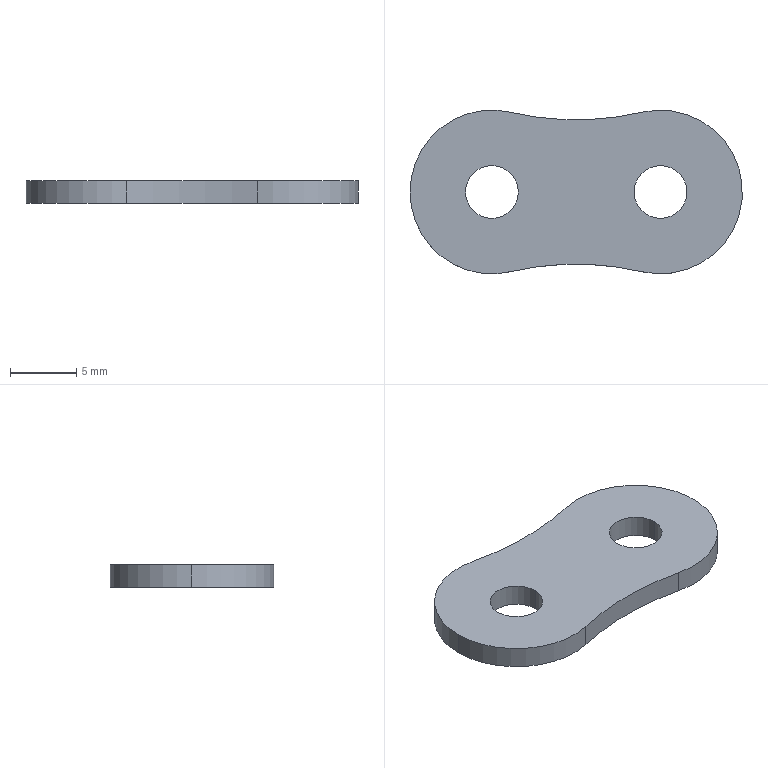Part | SolidWorks | features Cut 1, Extrusion 1 | 1 solid | 11 faces | box 25.03 x 12.33 x 1.665 mm | volume 399.679 mm3 | cylinder 9 | plane 2 | commonest cylinder face diameters 3.98 x4 12.33 x3 43.376 x2
STEP:
#1=CARTESIAN_POINT('',(4.36,0.,0.));
#2=VERTEX_POINT('',#1);
#3=CARTESIAN_POINT('',(8.34,0.,0.));
#4=VERTEX_POINT('',#3);
#5=CARTESIAN_POINT('',(6.35,0.,0.));
#6=DIRECTION('',(0.,0.,1.));
#7=DIRECTION('',(1.,0.,0.));
#8=AXIS2_PLACEMENT_3D('',#5,#6,#7);
#9=CIRCLE('',#8,1.99);
#10=EDGE_CURVE('',#2,#4,#9,.T.);
#11=ORIENTED_EDGE('',*,*,#10,.F.);
#12=CARTESIAN_POINT('',(4.36,0.,1.665));
#13=VERTEX_POINT('',#12);
#14=CARTESIAN_POINT('',(4.36,0.,0.));
#15=DIRECTION('',(0.,0.,1.));
#16=VECTOR('',#15,1000.);
#17=LINE('',#14,#16);
#18=EDGE_CURVE('',#2,#13,#17,.T.);
#19=ORIENTED_EDGE('',*,*,#18,.T.);
#20=CARTESIAN_POINT('',(8.34,0.,1.665));
#21=VERTEX_POINT('',#20);
#22=CARTESIAN_POINT('',(6.35,0.,1.665));
#23=DIRECTION('',(0.,0.,1.));
#24=DIRECTION('',(1.,0.,0.));
#25=AXIS2_PLACEMENT_3D('',#22,#23,#24);
#26=CIRCLE('',#25,1.99);
#27=EDGE_CURVE('',#13,#21,#26,.T.);
#28=ORIENTED_EDGE('',*,*,#27,.T.);
#29=CARTESIAN_POINT('',(8.34,0.,0.));
#30=DIRECTION('',(0.,0.,1.));
#31=VECTOR('',#30,1000.);
#32=LINE('',#29,#31);
#33=EDGE_CURVE('',#4,#21,#32,.T.);
#34=ORIENTED_EDGE('',*,*,#33,.F.);
#35=EDGE_LOOP('',(#11,#19,#28,#34));
#36=FACE_OUTER_BOUND('',#35,.T.);
#37=CARTESIAN_POINT('',(6.35,0.,0.));
#38=DIRECTION('',(0.,0.,1.));
#39=DIRECTION('',(1.,0.,0.));
#40=AXIS2_PLACEMENT_3D('',#37,#38,#39);
#41=CYLINDRICAL_SURFACE('',#40,1.99);
#42=ADVANCED_FACE('',(#36),#41,.F.);
#43=CARTESIAN_POINT('',(-8.34,0.,0.));
#44=VERTEX_POINT('',#43);
#45=CARTESIAN_POINT('',(-4.36,0.,0.));
#46=VERTEX_POINT('',#45);
#47=CARTESIAN_POINT('',(-6.35,0.,0.));
#48=DIRECTION('',(0.,0.,1.));
#49=DIRECTION('',(1.,0.,0.));
#50=AXIS2_PLACEMENT_3D('',#47,#48,#49);
#51=CIRCLE('',#50,1.99);
#52=EDGE_CURVE('',#44,#46,#51,.T.);
#53=ORIENTED_EDGE('',*,*,#52,.F.);
#54=CARTESIAN_POINT('',(-8.34,0.,1.665));
#55=VERTEX_POINT('',#54);
#56=CARTESIAN_POINT('',(-8.34,0.,0.));
#57=DIRECTION('',(0.,0.,1.));
#58=VECTOR('',#57,1000.);
#59=LINE('',#56,#58);
#60=EDGE_CURVE('',#44,#55,#59,.T.);
#61=ORIENTED_EDGE('',*,*,#60,.T.);
#62=CARTESIAN_POINT('',(-4.36,0.,1.665));
#63=VERTEX_POINT('',#62);
#64=CARTESIAN_POINT('',(-6.35,0.,1.665));
#65=DIRECTION('',(0.,0.,1.));
#66=DIRECTION('',(1.,0.,0.));
#67=AXIS2_PLACEMENT_3D('',#64,#65,#66);
#68=CIRCLE('',#67,1.99);
#69=EDGE_CURVE('',#55,#63,#68,.T.);
#70=ORIENTED_EDGE('',*,*,#69,.T.);
#71=CARTESIAN_POINT('',(-4.36,0.,0.));
#72=DIRECTION('',(0.,0.,1.));
#73=VECTOR('',#72,1000.);
#74=LINE('',#71,#73);
#75=EDGE_CURVE('',#46,#63,#74,.T.);
#76=ORIENTED_EDGE('',*,*,#75,.F.);
#77=EDGE_LOOP('',(#53,#61,#70,#76));
#78=FACE_OUTER_BOUND('',#77,.T.);
#79=CARTESIAN_POINT('',(-6.35,0.,0.));
#80=DIRECTION('',(0.,0.,1.));
#81=DIRECTION('',(1.,0.,0.));
#82=AXIS2_PLACEMENT_3D('',#79,#80,#81);
#83=CYLINDRICAL_SURFACE('',#82,1.99);
#84=ADVANCED_FACE('',(#78),#83,.F.);
#85=CARTESIAN_POINT('',(-12.515,0.,1.665));
#86=VERTEX_POINT('',#85);
#87=CARTESIAN_POINT('',(-4.944,-6.003,1.665));
#88=VERTEX_POINT('',#87);
#89=CARTESIAN_POINT('',(-6.35,0.,1.665));
#90=DIRECTION('',(0.,0.,1.));
#91=DIRECTION('',(1.,0.,0.));
#92=AXIS2_PLACEMENT_3D('',#89,#90,#91);
#93=CIRCLE('',#92,6.165);
#94=EDGE_CURVE('',#86,#88,#93,.T.);
#95=ORIENTED_EDGE('',*,*,#94,.F.);
#96=CARTESIAN_POINT('',(-12.515,0.,0.));
#97=VERTEX_POINT('',#96);
#98=CARTESIAN_POINT('',(-12.515,0.,1.665));
#99=DIRECTION('',(0.,0.,-1.));
#100=VECTOR('',#99,1000.);
#101=LINE('',#98,#100);
#102=EDGE_CURVE('',#86,#97,#101,.T.);
#103=ORIENTED_EDGE('',*,*,#102,.T.);
#104=CARTESIAN_POINT('',(-4.944,-6.003,0.));
#105=VERTEX_POINT('',#104);
#106=CARTESIAN_POINT('',(-6.35,0.,0.));
#107=DIRECTION('',(0.,0.,1.));
#108=DIRECTION('',(1.,0.,0.));
#109=AXIS2_PLACEMENT_3D('',#106,#107,#108);
#110=CIRCLE('',#109,6.165);
#111=EDGE_CURVE('',#97,#105,#110,.T.);
#112=ORIENTED_EDGE('',*,*,#111,.T.);
#113=CARTESIAN_POINT('',(-4.944,-6.003,1.665));
#114=DIRECTION('',(0.,0.,-1.));
#115=VECTOR('',#114,1000.);
#116=LINE('',#113,#115);
#117=EDGE_CURVE('',#88,#105,#116,.T.);
#118=ORIENTED_EDGE('',*,*,#117,.F.);
#119=EDGE_LOOP('',(#95,#103,#112,#118));
#120=FACE_OUTER_BOUND('',#119,.T.);
#121=CARTESIAN_POINT('',(-6.35,0.,1.665));
#122=DIRECTION('',(0.,0.,-1.));
#123=DIRECTION('',(-1.,0.,0.));
#124=AXIS2_PLACEMENT_3D('',#121,#122,#123);
#125=CYLINDRICAL_SURFACE('',#124,6.165);
#126=ADVANCED_FACE('',(#120),#125,.T.);
#127=CARTESIAN_POINT('',(4.944,-6.003,0.));
#128=VERTEX_POINT('',#127);
#129=CARTESIAN_POINT('',(0.,-27.12,0.));
#130=DIRECTION('',(0.,0.,-1.));
#131=DIRECTION('',(1.,0.,0.));
#132=AXIS2_PLACEMENT_3D('',#129,#130,#131);
#133=CIRCLE('',#132,21.688);
#134=EDGE_CURVE('',#105,#128,#133,.T.);
#135=ORIENTED_EDGE('',*,*,#134,.T.);
#136=CARTESIAN_POINT('',(4.944,-6.003,1.665));
#137=VERTEX_POINT('',#136);
#138=CARTESIAN_POINT('',(4.944,-6.003,1.665));
#139=DIRECTION('',(0.,0.,-1.));
#140=VECTOR('',#139,1000.);
#141=LINE('',#138,#140);
#142=EDGE_CURVE('',#137,#128,#141,.T.);
#143=ORIENTED_EDGE('',*,*,#142,.F.);
#144=CARTESIAN_POINT('',(0.,-27.12,1.665));
#145=DIRECTION('',(0.,0.,-1.));
#146=DIRECTION('',(1.,0.,0.));
#147=AXIS2_PLACEMENT_3D('',#144,#145,#146);
#148=CIRCLE('',#147,21.688);
#149=EDGE_CURVE('',#88,#137,#148,.T.);
#150=ORIENTED_EDGE('',*,*,#149,.F.);
#151=ORIENTED_EDGE('',*,*,#117,.T.);
#152=EDGE_LOOP('',(#135,#143,#150,#151));
#153=FACE_OUTER_BOUND('',#152,.T.);
#154=CARTESIAN_POINT('',(0.,-27.12,1.665));
#155=DIRECTION('',(0.,0.,-1.));
#156=DIRECTION('',(-1.,0.,0.));
#157=AXIS2_PLACEMENT_3D('',#154,#155,#156);
#158=CYLINDRICAL_SURFACE('',#157,21.688);
#159=ADVANCED_FACE('',(#153),#158,.F.);
#160=CARTESIAN_POINT('',(4.944,6.003,0.));
#161=VERTEX_POINT('',#160);
#162=CARTESIAN_POINT('',(6.35,0.,0.));
#163=DIRECTION('',(0.,0.,1.));
#164=DIRECTION('',(1.,0.,0.));
#165=AXIS2_PLACEMENT_3D('',#162,#163,#164);
#166=CIRCLE('',#165,6.165);
#167=EDGE_CURVE('',#128,#161,#166,.T.);
#168=ORIENTED_EDGE('',*,*,#167,.T.);
#169=CARTESIAN_POINT('',(4.944,6.003,1.665));
#170=VERTEX_POINT('',#169);
#171=CARTESIAN_POINT('',(4.944,6.003,1.665));
#172=DIRECTION('',(0.,0.,-1.));
#173=VECTOR('',#172,1000.);
#174=LINE('',#171,#173);
#175=EDGE_CURVE('',#170,#161,#174,.T.);
#176=ORIENTED_EDGE('',*,*,#175,.F.);
#177=CARTESIAN_POINT('',(6.35,0.,1.665));
#178=DIRECTION('',(0.,0.,1.));
#179=DIRECTION('',(1.,0.,0.));
#180=AXIS2_PLACEMENT_3D('',#177,#178,#179);
#181=CIRCLE('',#180,6.165);
#182=EDGE_CURVE('',#137,#170,#181,.T.);
#183=ORIENTED_EDGE('',*,*,#182,.F.);
#184=ORIENTED_EDGE('',*,*,#142,.T.);
#185=EDGE_LOOP('',(#168,#176,#183,#184));
#186=FACE_OUTER_BOUND('',#185,.T.);
#187=CARTESIAN_POINT('',(6.35,0.,1.665));
#188=DIRECTION('',(0.,0.,-1.));
#189=DIRECTION('',(-1.,0.,0.));
#190=AXIS2_PLACEMENT_3D('',#187,#188,#189);
#191=CYLINDRICAL_SURFACE('',#190,6.165);
#192=ADVANCED_FACE('',(#186),#191,.T.);
#193=CARTESIAN_POINT('',(-4.944,6.003,0.));
#194=VERTEX_POINT('',#193);
#195=CARTESIAN_POINT('',(0.,27.12,0.));
#196=DIRECTION('',(0.,0.,-1.));
#197=DIRECTION('',(1.,0.,0.));
#198=AXIS2_PLACEMENT_3D('',#195,#196,#197);
#199=CIRCLE('',#198,21.688);
#200=EDGE_CURVE('',#161,#194,#199,.T.);
#201=ORIENTED_EDGE('',*,*,#200,.T.);
#202=CARTESIAN_POINT('',(-4.944,6.003,1.665));
#203=VERTEX_POINT('',#202);
#204=CARTESIAN_POINT('',(-4.944,6.003,1.665));
#205=DIRECTION('',(0.,0.,-1.));
#206=VECTOR('',#205,1000.);
#207=LINE('',#204,#206);
#208=EDGE_CURVE('',#203,#194,#207,.T.);
#209=ORIENTED_EDGE('',*,*,#208,.F.);
#210=CARTESIAN_POINT('',(0.,27.12,1.665));
#211=DIRECTION('',(0.,0.,-1.));
#212=DIRECTION('',(1.,0.,0.));
#213=AXIS2_PLACEMENT_3D('',#210,#211,#212);
#214=CIRCLE('',#213,21.688);
#215=EDGE_CURVE('',#170,#203,#214,.T.);
#216=ORIENTED_EDGE('',*,*,#215,.F.);
#217=ORIENTED_EDGE('',*,*,#175,.T.);
#218=EDGE_LOOP('',(#201,#209,#216,#217));
#219=FACE_OUTER_BOUND('',#218,.T.);
#220=CARTESIAN_POINT('',(0.,27.12,1.665));
#221=DIRECTION('',(0.,0.,-1.));
#222=DIRECTION('',(-1.,0.,0.));
#223=AXIS2_PLACEMENT_3D('',#220,#221,#222);
#224=CYLINDRICAL_SURFACE('',#223,21.688);
#225=ADVANCED_FACE('',(#219),#224,.F.);
#226=ORIENTED_EDGE('',*,*,#102,.F.);
#227=CARTESIAN_POINT('',(-6.35,0.,1.665));
#228=DIRECTION('',(0.,0.,1.));
#229=DIRECTION('',(1.,0.,0.));
#230=AXIS2_PLACEMENT_3D('',#227,#228,#229);
#231=CIRCLE('',#230,6.165);
#232=EDGE_CURVE('',#203,#86,#231,.T.);
#233=ORIENTED_EDGE('',*,*,#232,.F.);
#234=ORIENTED_EDGE('',*,*,#208,.T.);
#235=CARTESIAN_POINT('',(-6.35,0.,0.));
#236=DIRECTION('',(0.,0.,1.));
#237=DIRECTION('',(1.,0.,0.));
#238=AXIS2_PLACEMENT_3D('',#235,#236,#237);
#239=CIRCLE('',#238,6.165);
#240=EDGE_CURVE('',#194,#97,#239,.T.);
#241=ORIENTED_EDGE('',*,*,#240,.T.);
#242=EDGE_LOOP('',(#226,#233,#234,#241));
#243=FACE_OUTER_BOUND('',#242,.T.);
#244=CARTESIAN_POINT('',(-6.35,0.,1.665));
#245=DIRECTION('',(0.,0.,-1.));
#246=DIRECTION('',(-1.,0.,0.));
#247=AXIS2_PLACEMENT_3D('',#244,#245,#246);
#248=CYLINDRICAL_SURFACE('',#247,6.165);
#249=ADVANCED_FACE('',(#243),#248,.T.);
#250=CARTESIAN_POINT('',(6.35,0.,1.665));
#251=DIRECTION('',(0.,0.,1.));
#252=DIRECTION('',(1.,0.,0.));
#253=AXIS2_PLACEMENT_3D('',#250,#251,#252);
#254=CIRCLE('',#253,1.99);
#255=EDGE_CURVE('',#21,#13,#254,.T.);
#256=ORIENTED_EDGE('',*,*,#255,.F.);
#257=ORIENTED_EDGE('',*,*,#27,.F.);
#258=EDGE_LOOP('',(#256,#257));
#259=FACE_BOUND('',#258,.T.);
#260=CARTESIAN_POINT('',(-6.35,0.,1.665));
#261=DIRECTION('',(0.,0.,1.));
#262=DIRECTION('',(1.,0.,0.));
#263=AXIS2_PLACEMENT_3D('',#260,#261,#262);
#264=CIRCLE('',#263,1.99);
#265=EDGE_CURVE('',#63,#55,#264,.T.);
#266=ORIENTED_EDGE('',*,*,#265,.F.);
#267=ORIENTED_EDGE('',*,*,#69,.F.);
#268=EDGE_LOOP('',(#266,#267));
#269=FACE_BOUND('',#268,.T.);
#270=ORIENTED_EDGE('',*,*,#149,.T.);
#271=ORIENTED_EDGE('',*,*,#182,.T.);
#272=ORIENTED_EDGE('',*,*,#215,.T.);
#273=ORIENTED_EDGE('',*,*,#232,.T.);
#274=ORIENTED_EDGE('',*,*,#94,.T.);
#275=EDGE_LOOP('',(#270,#271,#272,#273,#274));
#276=FACE_OUTER_BOUND('',#275,.T.);
#277=CARTESIAN_POINT('',(-3.175,-13.56,1.665));
#278=DIRECTION('',(0.,0.,1.));
#279=DIRECTION('',(1.,0.,0.));
#280=AXIS2_PLACEMENT_3D('',#277,#278,#279);
#281=PLANE('',#280);
#282=ADVANCED_FACE('',(#259,#269,#276),#281,.T.);
#283=CARTESIAN_POINT('',(6.35,0.,0.));
#284=DIRECTION('',(0.,0.,1.));
#285=DIRECTION('',(1.,0.,0.));
#286=AXIS2_PLACEMENT_3D('',#283,#284,#285);
#287=CIRCLE('',#286,1.99);
#288=EDGE_CURVE('',#4,#2,#287,.T.);
#289=ORIENTED_EDGE('',*,*,#288,.T.);
#290=ORIENTED_EDGE('',*,*,#10,.T.);
#291=EDGE_LOOP('',(#289,#290));
#292=FACE_BOUND('',#291,.T.);
#293=CARTESIAN_POINT('',(-6.35,0.,0.));
#294=DIRECTION('',(0.,0.,1.));
#295=DIRECTION('',(1.,0.,0.));
#296=AXIS2_PLACEMENT_3D('',#293,#294,#295);
#297=CIRCLE('',#296,1.99);
#298=EDGE_CURVE('',#46,#44,#297,.T.);
#299=ORIENTED_EDGE('',*,*,#298,.T.);
#300=ORIENTED_EDGE('',*,*,#52,.T.);
#301=EDGE_LOOP('',(#299,#300));
#302=FACE_BOUND('',#301,.T.);
#303=ORIENTED_EDGE('',*,*,#134,.F.);
#304=ORIENTED_EDGE('',*,*,#111,.F.);
#305=ORIENTED_EDGE('',*,*,#240,.F.);
#306=ORIENTED_EDGE('',*,*,#200,.F.);
#307=ORIENTED_EDGE('',*,*,#167,.F.);
#308=EDGE_LOOP('',(#303,#304,#305,#306,#307));
#309=FACE_OUTER_BOUND('',#308,.T.);
#310=CARTESIAN_POINT('',(-3.175,-13.56,0.));
#311=DIRECTION('',(0.,0.,1.));
#312=DIRECTION('',(1.,0.,0.));
#313=AXIS2_PLACEMENT_3D('',#310,#311,#312);
#314=PLANE('',#313);
#315=ADVANCED_FACE('',(#292,#302,#309),#314,.F.);
#316=ORIENTED_EDGE('',*,*,#60,.F.);
#317=ORIENTED_EDGE('',*,*,#298,.F.);
#318=ORIENTED_EDGE('',*,*,#75,.T.);
#319=ORIENTED_EDGE('',*,*,#265,.T.);
#320=EDGE_LOOP('',(#316,#317,#318,#319));
#321=FACE_OUTER_BOUND('',#320,.T.);
#322=CARTESIAN_POINT('',(-6.35,0.,0.));
#323=DIRECTION('',(0.,0.,1.));
#324=DIRECTION('',(1.,0.,0.));
#325=AXIS2_PLACEMENT_3D('',#322,#323,#324);
#326=CYLINDRICAL_SURFACE('',#325,1.99);
#327=ADVANCED_FACE('',(#321),#326,.F.);
#328=ORIENTED_EDGE('',*,*,#18,.F.);
#329=ORIENTED_EDGE('',*,*,#288,.F.);
#330=ORIENTED_EDGE('',*,*,#33,.T.);
#331=ORIENTED_EDGE('',*,*,#255,.T.);
#332=EDGE_LOOP('',(#328,#329,#330,#331));
#333=FACE_OUTER_BOUND('',#332,.T.);
#334=CARTESIAN_POINT('',(6.35,0.,0.));
#335=DIRECTION('',(0.,0.,1.));
#336=DIRECTION('',(1.,0.,0.));
#337=AXIS2_PLACEMENT_3D('',#334,#335,#336);
#338=CYLINDRICAL_SURFACE('',#337,1.99);
#339=ADVANCED_FACE('',(#333),#338,.F.);
#340=CLOSED_SHELL('',(#42,#84,#126,#159,#192,#225,#249,#282,#315,#327,#339));
#341=MANIFOLD_SOLID_BREP('',#340);
#342=CARTESIAN_POINT('',(0.,0.,0.));
#343=DIRECTION('',(0.,0.,1.));
#344=DIRECTION('',(1.,0.,0.));
#345=AXIS2_PLACEMENT_3D('',#342,#343,#344);
#346=(LENGTH_UNIT()NAMED_UNIT(*)SI_UNIT(.MILLI.,.METRE.));
#347=UNCERTAINTY_MEASURE_WITH_UNIT(LENGTH_MEASURE(0.00001),#346,'','');
#348=(NAMED_UNIT(*)PLANE_ANGLE_UNIT()SI_UNIT($,.RADIAN.));
#349=(NAMED_UNIT(*)SI_UNIT($,.STERADIAN.)SOLID_ANGLE_UNIT());
#350=(GEOMETRIC_REPRESENTATION_CONTEXT(3)GLOBAL_UNCERTAINTY_ASSIGNED_CONTEXT((#347))GLOBAL_UNIT_ASSIGNED_CONTEXT((#346,#348,#349))REPRESENTATION_CONTEXT('',''));
#351=ADVANCED_BREP_SHAPE_REPRESENTATION('',(#341,#345),#350);